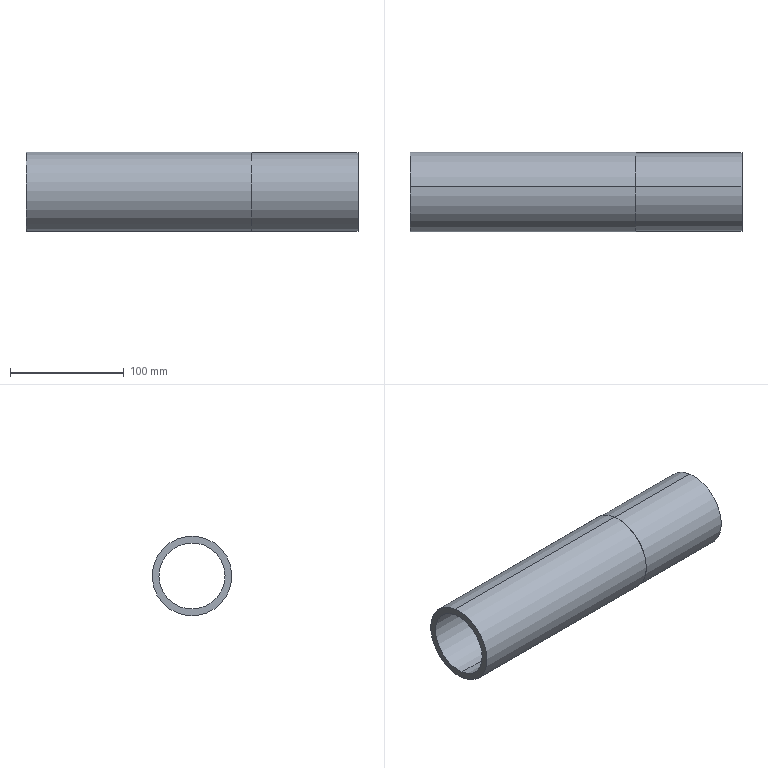Part | NX | features BREP 1 | 1 solid | 9 faces | box 291.64 x 70 x 70 mm | volume 341614 mm3 | cylinder 6 | plane 3 | commonest cylinder face diameters 58 x2 69 x2 70 x2
STEP:
#1=CARTESIAN_POINT('',(-58.925,3.913,28.735));
#2=VERTEX_POINT('',#1);
#3=CARTESIAN_POINT('',(-58.925,-3.913,-28.735));
#4=VERTEX_POINT('',#3);
#5=CARTESIAN_POINT('',(-58.925,0.,0.));
#6=DIRECTION('',(1.,0.,0.));
#7=DIRECTION('',(0.,-0.1349,-0.9909));
#8=AXIS2_PLACEMENT_3D('',#5,#6,#7);
#9=CIRCLE('',#8,29.);
#10=EDGE_CURVE('',#2,#4,#9,.T.);
#11=ORIENTED_EDGE('',*,*,#10,.T.);
#12=CARTESIAN_POINT('',(-350.565,-3.913,-28.735));
#13=VERTEX_POINT('',#12);
#14=CARTESIAN_POINT('',(-530.465,-3.913,-28.735));
#15=DIRECTION('',(-1.,0.,0.));
#16=VECTOR('',#15,1000.);
#17=LINE('',#14,#16);
#18=EDGE_CURVE('',#4,#13,#17,.T.);
#19=ORIENTED_EDGE('',*,*,#18,.T.);
#20=CARTESIAN_POINT('',(-350.565,3.913,28.735));
#21=VERTEX_POINT('',#20);
#22=CARTESIAN_POINT('',(-350.565,0.,0.));
#23=DIRECTION('',(-1.,0.,0.));
#24=DIRECTION('',(0.,0.,1.));
#25=AXIS2_PLACEMENT_3D('',#22,#23,#24);
#26=CIRCLE('',#25,29.);
#27=EDGE_CURVE('',#13,#21,#26,.T.);
#28=ORIENTED_EDGE('',*,*,#27,.T.);
#29=CARTESIAN_POINT('',(-530.465,3.913,28.735));
#30=DIRECTION('',(-1.,0.,0.));
#31=VECTOR('',#30,1000.);
#32=LINE('',#29,#31);
#33=EDGE_CURVE('',#2,#21,#32,.T.);
#34=ORIENTED_EDGE('',*,*,#33,.F.);
#35=EDGE_LOOP('',(#11,#19,#28,#34));
#36=FACE_BOUND('',#35,.T.);
#37=CARTESIAN_POINT('',(-530.465,0.,0.));
#38=DIRECTION('',(-1.,0.,0.));
#39=DIRECTION('',(0.,-0.1349,-0.9909));
#40=AXIS2_PLACEMENT_3D('',#37,#38,#39);
#41=CYLINDRICAL_SURFACE('',#40,29.);
#42=ADVANCED_FACE('',(#36),#41,.F.);
#43=CARTESIAN_POINT('',(-58.925,-4.655,-34.185));
#44=VERTEX_POINT('',#43);
#45=CARTESIAN_POINT('',(-58.925,4.655,34.185));
#46=VERTEX_POINT('',#45);
#47=CARTESIAN_POINT('',(-58.925,0.,0.));
#48=DIRECTION('',(1.,0.,0.));
#49=DIRECTION('',(0.,-0.1349,-0.9909));
#50=AXIS2_PLACEMENT_3D('',#47,#48,#49);
#51=CIRCLE('',#50,34.5);
#52=EDGE_CURVE('',#44,#46,#51,.T.);
#53=ORIENTED_EDGE('',*,*,#52,.F.);
#54=CARTESIAN_POINT('',(-152.465,-4.655,-34.185));
#55=VERTEX_POINT('',#54);
#56=CARTESIAN_POINT('',(-58.925,-4.655,-34.185));
#57=DIRECTION('',(-1.,0.,0.));
#58=VECTOR('',#57,1000.);
#59=LINE('',#56,#58);
#60=EDGE_CURVE('',#44,#55,#59,.T.);
#61=ORIENTED_EDGE('',*,*,#60,.T.);
#62=CARTESIAN_POINT('',(-152.465,4.655,34.185));
#63=VERTEX_POINT('',#62);
#64=CARTESIAN_POINT('',(-152.465,0.,0.));
#65=DIRECTION('',(1.,0.,0.));
#66=DIRECTION('',(0.,-0.1349,-0.9909));
#67=AXIS2_PLACEMENT_3D('',#64,#65,#66);
#68=CIRCLE('',#67,34.5);
#69=EDGE_CURVE('',#55,#63,#68,.T.);
#70=ORIENTED_EDGE('',*,*,#69,.T.);
#71=CARTESIAN_POINT('',(-58.925,4.655,34.185));
#72=DIRECTION('',(-1.,0.,0.));
#73=VECTOR('',#72,1000.);
#74=LINE('',#71,#73);
#75=EDGE_CURVE('',#46,#63,#74,.T.);
#76=ORIENTED_EDGE('',*,*,#75,.F.);
#77=EDGE_LOOP('',(#53,#61,#70,#76));
#78=FACE_BOUND('',#77,.T.);
#79=CARTESIAN_POINT('',(-58.925,0.,0.));
#80=DIRECTION('',(-1.,0.,0.));
#81=DIRECTION('',(0.,-0.1349,-0.9909));
#82=AXIS2_PLACEMENT_3D('',#79,#80,#81);
#83=CYLINDRICAL_SURFACE('',#82,34.5);
#84=ADVANCED_FACE('',(#78),#83,.T.);
#85=CARTESIAN_POINT('',(-152.465,4.722,34.68));
#86=VERTEX_POINT('',#85);
#87=CARTESIAN_POINT('',(-152.465,-4.722,-34.68));
#88=VERTEX_POINT('',#87);
#89=CARTESIAN_POINT('',(-152.465,0.,0.));
#90=DIRECTION('',(-1.,0.,0.));
#91=DIRECTION('',(0.,0.1349,0.9909));
#92=AXIS2_PLACEMENT_3D('',#89,#90,#91);
#93=CIRCLE('',#92,35.);
#94=EDGE_CURVE('',#86,#88,#93,.T.);
#95=ORIENTED_EDGE('',*,*,#94,.T.);
#96=CARTESIAN_POINT('',(-350.565,-4.722,-34.68));
#97=VERTEX_POINT('',#96);
#98=CARTESIAN_POINT('',(-530.465,-4.722,-34.68));
#99=DIRECTION('',(-1.,0.,0.));
#100=VECTOR('',#99,1000.);
#101=LINE('',#98,#100);
#102=EDGE_CURVE('',#88,#97,#101,.T.);
#103=ORIENTED_EDGE('',*,*,#102,.T.);
#104=CARTESIAN_POINT('',(-350.565,4.722,34.68));
#105=VERTEX_POINT('',#104);
#106=CARTESIAN_POINT('',(-350.565,0.,0.));
#107=DIRECTION('',(1.,0.,0.));
#108=DIRECTION('',(0.,0.,1.));
#109=AXIS2_PLACEMENT_3D('',#106,#107,#108);
#110=CIRCLE('',#109,35.);
#111=EDGE_CURVE('',#97,#105,#110,.T.);
#112=ORIENTED_EDGE('',*,*,#111,.T.);
#113=CARTESIAN_POINT('',(-530.465,4.722,34.68));
#114=DIRECTION('',(-1.,0.,0.));
#115=VECTOR('',#114,1000.);
#116=LINE('',#113,#115);
#117=EDGE_CURVE('',#86,#105,#116,.T.);
#118=ORIENTED_EDGE('',*,*,#117,.F.);
#119=EDGE_LOOP('',(#95,#103,#112,#118));
#120=FACE_BOUND('',#119,.T.);
#121=CARTESIAN_POINT('',(-530.465,0.,0.));
#122=DIRECTION('',(-1.,0.,0.));
#123=DIRECTION('',(0.,-0.1349,-0.9909));
#124=AXIS2_PLACEMENT_3D('',#121,#122,#123);
#125=CYLINDRICAL_SURFACE('',#124,35.);
#126=ADVANCED_FACE('',(#120),#125,.T.);
#127=CARTESIAN_POINT('',(-350.565,0.,0.));
#128=DIRECTION('',(-1.,0.,0.));
#129=DIRECTION('',(0.,0.,1.));
#130=AXIS2_PLACEMENT_3D('',#127,#128,#129);
#131=CIRCLE('',#130,29.);
#132=EDGE_CURVE('',#21,#13,#131,.T.);
#133=ORIENTED_EDGE('',*,*,#132,.F.);
#134=ORIENTED_EDGE('',*,*,#27,.F.);
#135=EDGE_LOOP('',(#133,#134));
#136=FACE_BOUND('',#135,.T.);
#137=CARTESIAN_POINT('',(-350.565,0.,0.));
#138=DIRECTION('',(1.,0.,0.));
#139=DIRECTION('',(0.,0.,1.));
#140=AXIS2_PLACEMENT_3D('',#137,#138,#139);
#141=CIRCLE('',#140,35.);
#142=EDGE_CURVE('',#105,#97,#141,.T.);
#143=ORIENTED_EDGE('',*,*,#142,.F.);
#144=ORIENTED_EDGE('',*,*,#111,.F.);
#145=EDGE_LOOP('',(#143,#144));
#146=FACE_BOUND('',#145,.T.);
#147=CARTESIAN_POINT('',(-350.565,0.,0.));
#148=DIRECTION('',(-1.,0.,0.));
#149=DIRECTION('',(0.,0.,-1.));
#150=AXIS2_PLACEMENT_3D('',#147,#148,#149);
#151=PLANE('',#150);
#152=ADVANCED_FACE('',(#136,#146),#151,.T.);
#153=CARTESIAN_POINT('',(-152.465,0.,0.));
#154=DIRECTION('',(1.,0.,0.));
#155=DIRECTION('',(0.,-0.1349,-0.9909));
#156=AXIS2_PLACEMENT_3D('',#153,#154,#155);
#157=CIRCLE('',#156,34.5);
#158=EDGE_CURVE('',#63,#55,#157,.T.);
#159=ORIENTED_EDGE('',*,*,#158,.F.);
#160=ORIENTED_EDGE('',*,*,#69,.F.);
#161=EDGE_LOOP('',(#159,#160));
#162=FACE_BOUND('',#161,.T.);
#163=ORIENTED_EDGE('',*,*,#94,.F.);
#164=CARTESIAN_POINT('',(-152.465,0.,0.));
#165=DIRECTION('',(-1.,0.,0.));
#166=DIRECTION('',(0.,0.1349,0.9909));
#167=AXIS2_PLACEMENT_3D('',#164,#165,#166);
#168=CIRCLE('',#167,35.);
#169=EDGE_CURVE('',#88,#86,#168,.T.);
#170=ORIENTED_EDGE('',*,*,#169,.F.);
#171=EDGE_LOOP('',(#163,#170));
#172=FACE_BOUND('',#171,.T.);
#173=CARTESIAN_POINT('',(-152.465,0.,0.));
#174=DIRECTION('',(-1.,0.,0.));
#175=DIRECTION('',(0.,-0.1349,-0.9909));
#176=AXIS2_PLACEMENT_3D('',#173,#174,#175);
#177=PLANE('',#176);
#178=ADVANCED_FACE('',(#162,#172),#177,.F.);
#179=ORIENTED_EDGE('',*,*,#102,.F.);
#180=ORIENTED_EDGE('',*,*,#169,.T.);
#181=ORIENTED_EDGE('',*,*,#117,.T.);
#182=ORIENTED_EDGE('',*,*,#142,.T.);
#183=EDGE_LOOP('',(#179,#180,#181,#182));
#184=FACE_BOUND('',#183,.T.);
#185=CARTESIAN_POINT('',(-530.465,0.,0.));
#186=DIRECTION('',(-1.,0.,0.));
#187=DIRECTION('',(0.,-0.1349,-0.9909));
#188=AXIS2_PLACEMENT_3D('',#185,#186,#187);
#189=CYLINDRICAL_SURFACE('',#188,35.);
#190=ADVANCED_FACE('',(#184),#189,.T.);
#191=ORIENTED_EDGE('',*,*,#60,.F.);
#192=CARTESIAN_POINT('',(-58.925,0.,0.));
#193=DIRECTION('',(1.,0.,0.));
#194=DIRECTION('',(0.,-0.1349,-0.9909));
#195=AXIS2_PLACEMENT_3D('',#192,#193,#194);
#196=CIRCLE('',#195,34.5);
#197=EDGE_CURVE('',#46,#44,#196,.T.);
#198=ORIENTED_EDGE('',*,*,#197,.F.);
#199=ORIENTED_EDGE('',*,*,#75,.T.);
#200=ORIENTED_EDGE('',*,*,#158,.T.);
#201=EDGE_LOOP('',(#191,#198,#199,#200));
#202=FACE_BOUND('',#201,.T.);
#203=CARTESIAN_POINT('',(-58.925,0.,0.));
#204=DIRECTION('',(-1.,0.,0.));
#205=DIRECTION('',(0.,-0.1349,-0.9909));
#206=AXIS2_PLACEMENT_3D('',#203,#204,#205);
#207=CYLINDRICAL_SURFACE('',#206,34.5);
#208=ADVANCED_FACE('',(#202),#207,.T.);
#209=ORIENTED_EDGE('',*,*,#10,.F.);
#210=CARTESIAN_POINT('',(-58.925,0.,0.));
#211=DIRECTION('',(1.,0.,0.));
#212=DIRECTION('',(0.,-0.1349,-0.9909));
#213=AXIS2_PLACEMENT_3D('',#210,#211,#212);
#214=CIRCLE('',#213,29.);
#215=EDGE_CURVE('',#4,#2,#214,.T.);
#216=ORIENTED_EDGE('',*,*,#215,.F.);
#217=EDGE_LOOP('',(#209,#216));
#218=FACE_BOUND('',#217,.T.);
#219=ORIENTED_EDGE('',*,*,#197,.T.);
#220=ORIENTED_EDGE('',*,*,#52,.T.);
#221=EDGE_LOOP('',(#219,#220));
#222=FACE_BOUND('',#221,.T.);
#223=CARTESIAN_POINT('',(-58.925,0.,0.));
#224=DIRECTION('',(1.,0.,0.));
#225=DIRECTION('',(0.,0.1349,0.9909));
#226=AXIS2_PLACEMENT_3D('',#223,#224,#225);
#227=PLANE('',#226);
#228=ADVANCED_FACE('',(#218,#222),#227,.T.);
#229=ORIENTED_EDGE('',*,*,#18,.F.);
#230=ORIENTED_EDGE('',*,*,#215,.T.);
#231=ORIENTED_EDGE('',*,*,#33,.T.);
#232=ORIENTED_EDGE('',*,*,#132,.T.);
#233=EDGE_LOOP('',(#229,#230,#231,#232));
#234=FACE_BOUND('',#233,.T.);
#235=CARTESIAN_POINT('',(-530.465,0.,0.));
#236=DIRECTION('',(-1.,0.,0.));
#237=DIRECTION('',(0.,-0.1349,-0.9909));
#238=AXIS2_PLACEMENT_3D('',#235,#236,#237);
#239=CYLINDRICAL_SURFACE('',#238,29.);
#240=ADVANCED_FACE('',(#234),#239,.F.);
#241=CLOSED_SHELL('',(#42,#84,#126,#152,#178,#190,#208,#228,#240));
#242=MANIFOLD_SOLID_BREP('',#241);
#243=(LENGTH_UNIT()NAMED_UNIT(*)SI_UNIT(.MILLI.,.METRE.));
#244=UNCERTAINTY_MEASURE_WITH_UNIT(LENGTH_MEASURE(0.00001),#243,'','');
#245=(NAMED_UNIT(*)PLANE_ANGLE_UNIT()SI_UNIT($,.RADIAN.));
#246=(NAMED_UNIT(*)SI_UNIT($,.STERADIAN.)SOLID_ANGLE_UNIT());
#247=(GEOMETRIC_REPRESENTATION_CONTEXT(3)GLOBAL_UNCERTAINTY_ASSIGNED_CONTEXT((#244))GLOBAL_UNIT_ASSIGNED_CONTEXT((#243,#245,#246))REPRESENTATION_CONTEXT('',''));
#248=ADVANCED_BREP_SHAPE_REPRESENTATION('',(#242),#247);